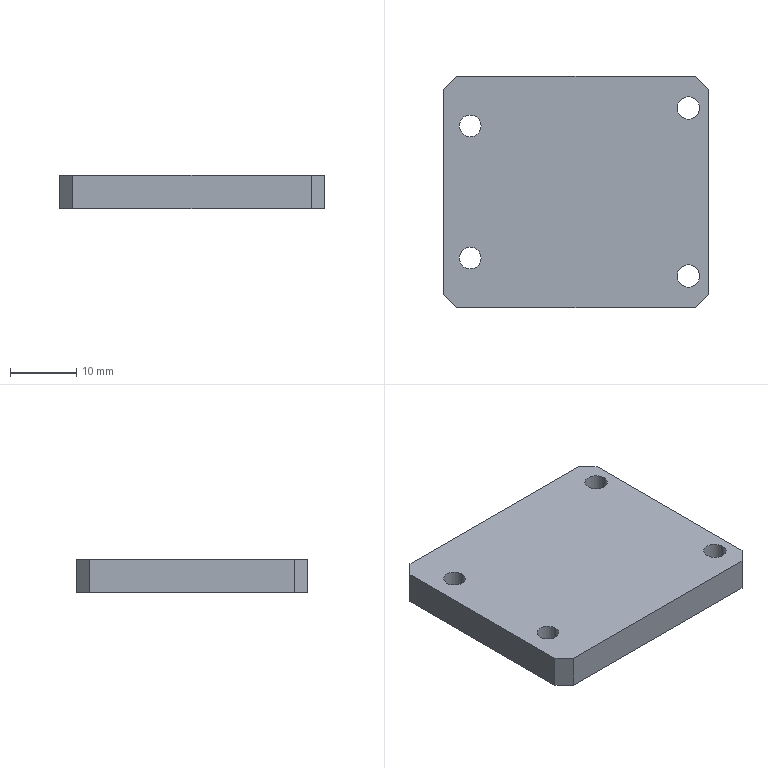Part | SolidWorks | features BaseBody 1 | 1 solid | 18 faces | box 40 x 35 x 5 mm | volume 6784 mm3 | plane 10 | cylinder 8 | commonest cylinder face diameters 3.3 x4 3.4 x4
STEP:
#1=CARTESIAN_POINT('',(18.7,12.7,5.));
#2=VERTEX_POINT('',#1);
#3=CARTESIAN_POINT('',(15.3,12.7,5.));
#4=VERTEX_POINT('',#3);
#5=CARTESIAN_POINT('',(17.,12.7,5.));
#6=DIRECTION('',(0.,0.,-1.));
#7=DIRECTION('',(-1.,0.,0.));
#8=AXIS2_PLACEMENT_3D('',#5,#6,#7);
#9=CIRCLE('',#8,1.7);
#10=EDGE_CURVE('',#2,#4,#9,.T.);
#11=ORIENTED_EDGE('',*,*,#10,.F.);
#12=CARTESIAN_POINT('',(18.7,12.7,0.));
#13=VERTEX_POINT('',#12);
#14=CARTESIAN_POINT('',(18.7,12.7,0.));
#15=DIRECTION('',(0.,0.,-1.));
#16=VECTOR('',#15,1000.);
#17=LINE('',#14,#16);
#18=EDGE_CURVE('',#2,#13,#17,.T.);
#19=ORIENTED_EDGE('',*,*,#18,.T.);
#20=CARTESIAN_POINT('',(15.3,12.7,0.));
#21=VERTEX_POINT('',#20);
#22=CARTESIAN_POINT('',(17.,12.7,0.));
#23=DIRECTION('',(0.,0.,-1.));
#24=DIRECTION('',(-1.,0.,0.));
#25=AXIS2_PLACEMENT_3D('',#22,#23,#24);
#26=CIRCLE('',#25,1.7);
#27=EDGE_CURVE('',#13,#21,#26,.T.);
#28=ORIENTED_EDGE('',*,*,#27,.T.);
#29=CARTESIAN_POINT('',(15.3,12.7,0.));
#30=DIRECTION('',(0.,0.,-1.));
#31=VECTOR('',#30,1000.);
#32=LINE('',#29,#31);
#33=EDGE_CURVE('',#4,#21,#32,.T.);
#34=ORIENTED_EDGE('',*,*,#33,.F.);
#35=EDGE_LOOP('',(#11,#19,#28,#34));
#36=FACE_OUTER_BOUND('',#35,.T.);
#37=CARTESIAN_POINT('',(17.,12.7,0.));
#38=DIRECTION('',(0.,0.,-1.));
#39=DIRECTION('',(-1.,0.,0.));
#40=AXIS2_PLACEMENT_3D('',#37,#38,#39);
#41=CYLINDRICAL_SURFACE('',#40,1.7);
#42=ADVANCED_FACE('',(#36),#41,.F.);
#43=CARTESIAN_POINT('',(18.7,-12.7,5.));
#44=VERTEX_POINT('',#43);
#45=CARTESIAN_POINT('',(15.3,-12.7,5.));
#46=VERTEX_POINT('',#45);
#47=CARTESIAN_POINT('',(17.,-12.7,5.));
#48=DIRECTION('',(0.,0.,-1.));
#49=DIRECTION('',(-1.,0.,0.));
#50=AXIS2_PLACEMENT_3D('',#47,#48,#49);
#51=CIRCLE('',#50,1.7);
#52=EDGE_CURVE('',#44,#46,#51,.T.);
#53=ORIENTED_EDGE('',*,*,#52,.F.);
#54=CARTESIAN_POINT('',(18.7,-12.7,0.));
#55=VERTEX_POINT('',#54);
#56=CARTESIAN_POINT('',(18.7,-12.7,0.));
#57=DIRECTION('',(0.,0.,-1.));
#58=VECTOR('',#57,1000.);
#59=LINE('',#56,#58);
#60=EDGE_CURVE('',#44,#55,#59,.T.);
#61=ORIENTED_EDGE('',*,*,#60,.T.);
#62=CARTESIAN_POINT('',(15.3,-12.7,0.));
#63=VERTEX_POINT('',#62);
#64=CARTESIAN_POINT('',(17.,-12.7,0.));
#65=DIRECTION('',(0.,0.,-1.));
#66=DIRECTION('',(-1.,0.,0.));
#67=AXIS2_PLACEMENT_3D('',#64,#65,#66);
#68=CIRCLE('',#67,1.7);
#69=EDGE_CURVE('',#55,#63,#68,.T.);
#70=ORIENTED_EDGE('',*,*,#69,.T.);
#71=CARTESIAN_POINT('',(15.3,-12.7,0.));
#72=DIRECTION('',(0.,0.,-1.));
#73=VECTOR('',#72,1000.);
#74=LINE('',#71,#73);
#75=EDGE_CURVE('',#46,#63,#74,.T.);
#76=ORIENTED_EDGE('',*,*,#75,.F.);
#77=EDGE_LOOP('',(#53,#61,#70,#76));
#78=FACE_OUTER_BOUND('',#77,.T.);
#79=CARTESIAN_POINT('',(17.,-12.7,0.));
#80=DIRECTION('',(0.,0.,-1.));
#81=DIRECTION('',(-1.,0.,0.));
#82=AXIS2_PLACEMENT_3D('',#79,#80,#81);
#83=CYLINDRICAL_SURFACE('',#82,1.7);
#84=ADVANCED_FACE('',(#78),#83,.F.);
#85=CARTESIAN_POINT('',(-14.35,10.,5.));
#86=VERTEX_POINT('',#85);
#87=CARTESIAN_POINT('',(-17.65,10.,5.));
#88=VERTEX_POINT('',#87);
#89=CARTESIAN_POINT('',(-16.,10.,5.));
#90=DIRECTION('',(0.,0.,-1.));
#91=DIRECTION('',(-1.,0.,0.));
#92=AXIS2_PLACEMENT_3D('',#89,#90,#91);
#93=CIRCLE('',#92,1.65);
#94=EDGE_CURVE('',#86,#88,#93,.T.);
#95=ORIENTED_EDGE('',*,*,#94,.F.);
#96=CARTESIAN_POINT('',(-14.35,10.,0.));
#97=VERTEX_POINT('',#96);
#98=CARTESIAN_POINT('',(-14.35,10.,0.));
#99=DIRECTION('',(0.,0.,-1.));
#100=VECTOR('',#99,1000.);
#101=LINE('',#98,#100);
#102=EDGE_CURVE('',#86,#97,#101,.T.);
#103=ORIENTED_EDGE('',*,*,#102,.T.);
#104=CARTESIAN_POINT('',(-17.65,10.,0.));
#105=VERTEX_POINT('',#104);
#106=CARTESIAN_POINT('',(-16.,10.,0.));
#107=DIRECTION('',(0.,0.,-1.));
#108=DIRECTION('',(-1.,0.,0.));
#109=AXIS2_PLACEMENT_3D('',#106,#107,#108);
#110=CIRCLE('',#109,1.65);
#111=EDGE_CURVE('',#97,#105,#110,.T.);
#112=ORIENTED_EDGE('',*,*,#111,.T.);
#113=CARTESIAN_POINT('',(-17.65,10.,0.));
#114=DIRECTION('',(0.,0.,-1.));
#115=VECTOR('',#114,1000.);
#116=LINE('',#113,#115);
#117=EDGE_CURVE('',#88,#105,#116,.T.);
#118=ORIENTED_EDGE('',*,*,#117,.F.);
#119=EDGE_LOOP('',(#95,#103,#112,#118));
#120=FACE_OUTER_BOUND('',#119,.T.);
#121=CARTESIAN_POINT('',(-16.,10.,0.));
#122=DIRECTION('',(0.,0.,-1.));
#123=DIRECTION('',(-1.,0.,0.));
#124=AXIS2_PLACEMENT_3D('',#121,#122,#123);
#125=CYLINDRICAL_SURFACE('',#124,1.65);
#126=ADVANCED_FACE('',(#120),#125,.F.);
#127=CARTESIAN_POINT('',(-14.35,-10.,5.));
#128=VERTEX_POINT('',#127);
#129=CARTESIAN_POINT('',(-17.65,-10.,5.));
#130=VERTEX_POINT('',#129);
#131=CARTESIAN_POINT('',(-16.,-10.,5.));
#132=DIRECTION('',(0.,0.,-1.));
#133=DIRECTION('',(-1.,0.,0.));
#134=AXIS2_PLACEMENT_3D('',#131,#132,#133);
#135=CIRCLE('',#134,1.65);
#136=EDGE_CURVE('',#128,#130,#135,.T.);
#137=ORIENTED_EDGE('',*,*,#136,.F.);
#138=CARTESIAN_POINT('',(-14.35,-10.,0.));
#139=VERTEX_POINT('',#138);
#140=CARTESIAN_POINT('',(-14.35,-10.,0.));
#141=DIRECTION('',(0.,0.,-1.));
#142=VECTOR('',#141,1000.);
#143=LINE('',#140,#142);
#144=EDGE_CURVE('',#128,#139,#143,.T.);
#145=ORIENTED_EDGE('',*,*,#144,.T.);
#146=CARTESIAN_POINT('',(-17.65,-10.,0.));
#147=VERTEX_POINT('',#146);
#148=CARTESIAN_POINT('',(-16.,-10.,0.));
#149=DIRECTION('',(0.,0.,-1.));
#150=DIRECTION('',(-1.,0.,0.));
#151=AXIS2_PLACEMENT_3D('',#148,#149,#150);
#152=CIRCLE('',#151,1.65);
#153=EDGE_CURVE('',#139,#147,#152,.T.);
#154=ORIENTED_EDGE('',*,*,#153,.T.);
#155=CARTESIAN_POINT('',(-17.65,-10.,0.));
#156=DIRECTION('',(0.,0.,-1.));
#157=VECTOR('',#156,1000.);
#158=LINE('',#155,#157);
#159=EDGE_CURVE('',#130,#147,#158,.T.);
#160=ORIENTED_EDGE('',*,*,#159,.F.);
#161=EDGE_LOOP('',(#137,#145,#154,#160));
#162=FACE_OUTER_BOUND('',#161,.T.);
#163=CARTESIAN_POINT('',(-16.,-10.,0.));
#164=DIRECTION('',(0.,0.,-1.));
#165=DIRECTION('',(-1.,0.,0.));
#166=AXIS2_PLACEMENT_3D('',#163,#164,#165);
#167=CYLINDRICAL_SURFACE('',#166,1.65);
#168=ADVANCED_FACE('',(#162),#167,.F.);
#169=CARTESIAN_POINT('',(-20.,15.5,0.));
#170=VERTEX_POINT('',#169);
#171=CARTESIAN_POINT('',(-20.,-15.5,0.));
#172=VERTEX_POINT('',#171);
#173=CARTESIAN_POINT('',(-20.,17.5,0.));
#174=DIRECTION('',(0.,-1.,0.));
#175=VECTOR('',#174,1000.);
#176=LINE('',#173,#175);
#177=EDGE_CURVE('',#170,#172,#176,.T.);
#178=ORIENTED_EDGE('',*,*,#177,.T.);
#179=CARTESIAN_POINT('',(-20.,-15.5,5.));
#180=VERTEX_POINT('',#179);
#181=CARTESIAN_POINT('',(-20.,-15.5,5.));
#182=DIRECTION('',(0.,0.,1.));
#183=VECTOR('',#182,1000.);
#184=LINE('',#181,#183);
#185=EDGE_CURVE('',#172,#180,#184,.T.);
#186=ORIENTED_EDGE('',*,*,#185,.T.);
#187=CARTESIAN_POINT('',(-20.,15.5,5.));
#188=VERTEX_POINT('',#187);
#189=CARTESIAN_POINT('',(-20.,17.5,5.));
#190=DIRECTION('',(0.,-1.,0.));
#191=VECTOR('',#190,1000.);
#192=LINE('',#189,#191);
#193=EDGE_CURVE('',#188,#180,#192,.T.);
#194=ORIENTED_EDGE('',*,*,#193,.F.);
#195=CARTESIAN_POINT('',(-20.,15.5,5.));
#196=DIRECTION('',(0.,0.,-1.));
#197=VECTOR('',#196,1000.);
#198=LINE('',#195,#197);
#199=EDGE_CURVE('',#188,#170,#198,.T.);
#200=ORIENTED_EDGE('',*,*,#199,.T.);
#201=EDGE_LOOP('',(#178,#186,#194,#200));
#202=FACE_OUTER_BOUND('',#201,.T.);
#203=CARTESIAN_POINT('',(-20.,17.5,5.));
#204=DIRECTION('',(1.,0.,0.));
#205=DIRECTION('',(0.,1.,0.));
#206=AXIS2_PLACEMENT_3D('',#203,#204,#205);
#207=PLANE('',#206);
#208=ADVANCED_FACE('',(#202),#207,.F.);
#209=CARTESIAN_POINT('',(-18.,-17.5,0.));
#210=VERTEX_POINT('',#209);
#211=CARTESIAN_POINT('',(18.,-17.5,0.));
#212=VERTEX_POINT('',#211);
#213=CARTESIAN_POINT('',(20.,-17.5,0.));
#214=DIRECTION('',(1.,0.,0.));
#215=VECTOR('',#214,1000.);
#216=LINE('',#213,#215);
#217=EDGE_CURVE('',#210,#212,#216,.T.);
#218=ORIENTED_EDGE('',*,*,#217,.T.);
#219=CARTESIAN_POINT('',(18.,-17.5,5.));
#220=VERTEX_POINT('',#219);
#221=CARTESIAN_POINT('',(18.,-17.5,5.));
#222=DIRECTION('',(0.,0.,1.));
#223=VECTOR('',#222,1000.);
#224=LINE('',#221,#223);
#225=EDGE_CURVE('',#212,#220,#224,.T.);
#226=ORIENTED_EDGE('',*,*,#225,.T.);
#227=CARTESIAN_POINT('',(-18.,-17.5,5.));
#228=VERTEX_POINT('',#227);
#229=CARTESIAN_POINT('',(20.,-17.5,5.));
#230=DIRECTION('',(1.,0.,0.));
#231=VECTOR('',#230,1000.);
#232=LINE('',#229,#231);
#233=EDGE_CURVE('',#228,#220,#232,.T.);
#234=ORIENTED_EDGE('',*,*,#233,.F.);
#235=CARTESIAN_POINT('',(-18.,-17.5,5.));
#236=DIRECTION('',(0.,0.,-1.));
#237=VECTOR('',#236,1000.);
#238=LINE('',#235,#237);
#239=EDGE_CURVE('',#228,#210,#238,.T.);
#240=ORIENTED_EDGE('',*,*,#239,.T.);
#241=EDGE_LOOP('',(#218,#226,#234,#240));
#242=FACE_OUTER_BOUND('',#241,.T.);
#243=CARTESIAN_POINT('',(20.,-17.5,5.));
#244=DIRECTION('',(0.,1.,0.));
#245=DIRECTION('',(-1.,0.,0.));
#246=AXIS2_PLACEMENT_3D('',#243,#244,#245);
#247=PLANE('',#246);
#248=ADVANCED_FACE('',(#242),#247,.F.);
#249=CARTESIAN_POINT('',(20.,-15.5,5.));
#250=VERTEX_POINT('',#249);
#251=CARTESIAN_POINT('',(20.,15.5,5.));
#252=VERTEX_POINT('',#251);
#253=CARTESIAN_POINT('',(20.,17.5,5.));
#254=DIRECTION('',(0.,1.,0.));
#255=VECTOR('',#254,1000.);
#256=LINE('',#253,#255);
#257=EDGE_CURVE('',#250,#252,#256,.T.);
#258=ORIENTED_EDGE('',*,*,#257,.F.);
#259=CARTESIAN_POINT('',(20.,-15.5,0.));
#260=VERTEX_POINT('',#259);
#261=CARTESIAN_POINT('',(20.,-15.5,5.));
#262=DIRECTION('',(0.,0.,-1.));
#263=VECTOR('',#262,1000.);
#264=LINE('',#261,#263);
#265=EDGE_CURVE('',#250,#260,#264,.T.);
#266=ORIENTED_EDGE('',*,*,#265,.T.);
#267=CARTESIAN_POINT('',(20.,15.5,0.));
#268=VERTEX_POINT('',#267);
#269=CARTESIAN_POINT('',(20.,17.5,0.));
#270=DIRECTION('',(0.,1.,0.));
#271=VECTOR('',#270,1000.);
#272=LINE('',#269,#271);
#273=EDGE_CURVE('',#260,#268,#272,.T.);
#274=ORIENTED_EDGE('',*,*,#273,.T.);
#275=CARTESIAN_POINT('',(20.,15.5,5.));
#276=DIRECTION('',(0.,0.,1.));
#277=VECTOR('',#276,1000.);
#278=LINE('',#275,#277);
#279=EDGE_CURVE('',#268,#252,#278,.T.);
#280=ORIENTED_EDGE('',*,*,#279,.T.);
#281=EDGE_LOOP('',(#258,#266,#274,#280));
#282=FACE_OUTER_BOUND('',#281,.T.);
#283=CARTESIAN_POINT('',(20.,17.5,5.));
#284=DIRECTION('',(-1.,0.,0.));
#285=DIRECTION('',(0.,-1.,0.));
#286=AXIS2_PLACEMENT_3D('',#283,#284,#285);
#287=PLANE('',#286);
#288=ADVANCED_FACE('',(#282),#287,.F.);
#289=CARTESIAN_POINT('',(18.,17.5,5.));
#290=VERTEX_POINT('',#289);
#291=CARTESIAN_POINT('',(-18.,17.5,5.));
#292=VERTEX_POINT('',#291);
#293=CARTESIAN_POINT('',(20.,17.5,5.));
#294=DIRECTION('',(-1.,0.,0.));
#295=VECTOR('',#294,1000.);
#296=LINE('',#293,#295);
#297=EDGE_CURVE('',#290,#292,#296,.T.);
#298=ORIENTED_EDGE('',*,*,#297,.F.);
#299=CARTESIAN_POINT('',(18.,17.5,0.));
#300=VERTEX_POINT('',#299);
#301=CARTESIAN_POINT('',(18.,17.5,5.));
#302=DIRECTION('',(0.,0.,-1.));
#303=VECTOR('',#302,1000.);
#304=LINE('',#301,#303);
#305=EDGE_CURVE('',#290,#300,#304,.T.);
#306=ORIENTED_EDGE('',*,*,#305,.T.);
#307=CARTESIAN_POINT('',(-18.,17.5,0.));
#308=VERTEX_POINT('',#307);
#309=CARTESIAN_POINT('',(20.,17.5,0.));
#310=DIRECTION('',(-1.,0.,0.));
#311=VECTOR('',#310,1000.);
#312=LINE('',#309,#311);
#313=EDGE_CURVE('',#300,#308,#312,.T.);
#314=ORIENTED_EDGE('',*,*,#313,.T.);
#315=CARTESIAN_POINT('',(-18.,17.5,5.));
#316=DIRECTION('',(0.,0.,1.));
#317=VECTOR('',#316,1000.);
#318=LINE('',#315,#317);
#319=EDGE_CURVE('',#308,#292,#318,.T.);
#320=ORIENTED_EDGE('',*,*,#319,.T.);
#321=EDGE_LOOP('',(#298,#306,#314,#320));
#322=FACE_OUTER_BOUND('',#321,.T.);
#323=CARTESIAN_POINT('',(20.,17.5,5.));
#324=DIRECTION('',(0.,-1.,0.));
#325=DIRECTION('',(1.,0.,0.));
#326=AXIS2_PLACEMENT_3D('',#323,#324,#325);
#327=PLANE('',#326);
#328=ADVANCED_FACE('',(#322),#327,.F.);
#329=CARTESIAN_POINT('',(17.,12.7,5.));
#330=DIRECTION('',(0.,0.,-1.));
#331=DIRECTION('',(-1.,0.,0.));
#332=AXIS2_PLACEMENT_3D('',#329,#330,#331);
#333=CIRCLE('',#332,1.7);
#334=EDGE_CURVE('',#4,#2,#333,.T.);
#335=ORIENTED_EDGE('',*,*,#334,.T.);
#336=ORIENTED_EDGE('',*,*,#10,.T.);
#337=EDGE_LOOP('',(#335,#336));
#338=FACE_BOUND('',#337,.T.);
#339=CARTESIAN_POINT('',(17.,-12.7,5.));
#340=DIRECTION('',(0.,0.,-1.));
#341=DIRECTION('',(-1.,0.,0.));
#342=AXIS2_PLACEMENT_3D('',#339,#340,#341);
#343=CIRCLE('',#342,1.7);
#344=EDGE_CURVE('',#46,#44,#343,.T.);
#345=ORIENTED_EDGE('',*,*,#344,.T.);
#346=ORIENTED_EDGE('',*,*,#52,.T.);
#347=EDGE_LOOP('',(#345,#346));
#348=FACE_BOUND('',#347,.T.);
#349=CARTESIAN_POINT('',(-16.,10.,5.));
#350=DIRECTION('',(0.,0.,-1.));
#351=DIRECTION('',(-1.,0.,0.));
#352=AXIS2_PLACEMENT_3D('',#349,#350,#351);
#353=CIRCLE('',#352,1.65);
#354=EDGE_CURVE('',#88,#86,#353,.T.);
#355=ORIENTED_EDGE('',*,*,#354,.T.);
#356=ORIENTED_EDGE('',*,*,#94,.T.);
#357=EDGE_LOOP('',(#355,#356));
#358=FACE_BOUND('',#357,.T.);
#359=CARTESIAN_POINT('',(-16.,-10.,5.));
#360=DIRECTION('',(0.,0.,-1.));
#361=DIRECTION('',(-1.,0.,0.));
#362=AXIS2_PLACEMENT_3D('',#359,#360,#361);
#363=CIRCLE('',#362,1.65);
#364=EDGE_CURVE('',#130,#128,#363,.T.);
#365=ORIENTED_EDGE('',*,*,#364,.T.);
#366=ORIENTED_EDGE('',*,*,#136,.T.);
#367=EDGE_LOOP('',(#365,#366));
#368=FACE_BOUND('',#367,.T.);
#369=ORIENTED_EDGE('',*,*,#233,.T.);
#370=CARTESIAN_POINT('',(20.,-15.5,5.));
#371=DIRECTION('',(0.7071,0.7071,0.));
#372=VECTOR('',#371,1000.);
#373=LINE('',#370,#372);
#374=EDGE_CURVE('',#220,#250,#373,.T.);
#375=ORIENTED_EDGE('',*,*,#374,.T.);
#376=ORIENTED_EDGE('',*,*,#257,.T.);
#377=CARTESIAN_POINT('',(18.,17.5,5.));
#378=DIRECTION('',(-0.7071,0.7071,0.));
#379=VECTOR('',#378,1000.);
#380=LINE('',#377,#379);
#381=EDGE_CURVE('',#252,#290,#380,.T.);
#382=ORIENTED_EDGE('',*,*,#381,.T.);
#383=ORIENTED_EDGE('',*,*,#297,.T.);
#384=CARTESIAN_POINT('',(-20.,15.5,5.));
#385=DIRECTION('',(-0.7071,-0.7071,0.));
#386=VECTOR('',#385,1000.);
#387=LINE('',#384,#386);
#388=EDGE_CURVE('',#292,#188,#387,.T.);
#389=ORIENTED_EDGE('',*,*,#388,.T.);
#390=ORIENTED_EDGE('',*,*,#193,.T.);
#391=CARTESIAN_POINT('',(-18.,-17.5,5.));
#392=DIRECTION('',(0.7071,-0.7071,0.));
#393=VECTOR('',#392,1000.);
#394=LINE('',#391,#393);
#395=EDGE_CURVE('',#180,#228,#394,.T.);
#396=ORIENTED_EDGE('',*,*,#395,.T.);
#397=EDGE_LOOP('',(#369,#375,#376,#382,#383,#389,#390,#396));
#398=FACE_OUTER_BOUND('',#397,.T.);
#399=CARTESIAN_POINT('',(0.,0.,5.));
#400=DIRECTION('',(0.,0.,-1.));
#401=DIRECTION('',(-1.,0.,0.));
#402=AXIS2_PLACEMENT_3D('',#399,#400,#401);
#403=PLANE('',#402);
#404=ADVANCED_FACE('',(#338,#348,#358,#368,#398),#403,.F.);
#405=CARTESIAN_POINT('',(17.,12.7,0.));
#406=DIRECTION('',(0.,0.,-1.));
#407=DIRECTION('',(-1.,0.,0.));
#408=AXIS2_PLACEMENT_3D('',#405,#406,#407);
#409=CIRCLE('',#408,1.7);
#410=EDGE_CURVE('',#21,#13,#409,.T.);
#411=ORIENTED_EDGE('',*,*,#410,.F.);
#412=ORIENTED_EDGE('',*,*,#27,.F.);
#413=EDGE_LOOP('',(#411,#412));
#414=FACE_BOUND('',#413,.T.);
#415=CARTESIAN_POINT('',(17.,-12.7,0.));
#416=DIRECTION('',(0.,0.,-1.));
#417=DIRECTION('',(-1.,0.,0.));
#418=AXIS2_PLACEMENT_3D('',#415,#416,#417);
#419=CIRCLE('',#418,1.7);
#420=EDGE_CURVE('',#63,#55,#419,.T.);
#421=ORIENTED_EDGE('',*,*,#420,.F.);
#422=ORIENTED_EDGE('',*,*,#69,.F.);
#423=EDGE_LOOP('',(#421,#422));
#424=FACE_BOUND('',#423,.T.);
#425=CARTESIAN_POINT('',(-16.,10.,0.));
#426=DIRECTION('',(0.,0.,-1.));
#427=DIRECTION('',(-1.,0.,0.));
#428=AXIS2_PLACEMENT_3D('',#425,#426,#427);
#429=CIRCLE('',#428,1.65);
#430=EDGE_CURVE('',#105,#97,#429,.T.);
#431=ORIENTED_EDGE('',*,*,#430,.F.);
#432=ORIENTED_EDGE('',*,*,#111,.F.);
#433=EDGE_LOOP('',(#431,#432));
#434=FACE_BOUND('',#433,.T.);
#435=CARTESIAN_POINT('',(-16.,-10.,0.));
#436=DIRECTION('',(0.,0.,-1.));
#437=DIRECTION('',(-1.,0.,0.));
#438=AXIS2_PLACEMENT_3D('',#435,#436,#437);
#439=CIRCLE('',#438,1.65);
#440=EDGE_CURVE('',#147,#139,#439,.T.);
#441=ORIENTED_EDGE('',*,*,#440,.F.);
#442=ORIENTED_EDGE('',*,*,#153,.F.);
#443=EDGE_LOOP('',(#441,#442));
#444=FACE_BOUND('',#443,.T.);
#445=ORIENTED_EDGE('',*,*,#273,.F.);
#446=CARTESIAN_POINT('',(17.75,-17.75,0.));
#447=DIRECTION('',(-0.7071,-0.7071,0.));
#448=VECTOR('',#447,1000.);
#449=LINE('',#446,#448);
#450=EDGE_CURVE('',#260,#212,#449,.T.);
#451=ORIENTED_EDGE('',*,*,#450,.T.);
#452=ORIENTED_EDGE('',*,*,#217,.F.);
#453=CARTESIAN_POINT('',(-17.75,-17.75,0.));
#454=DIRECTION('',(-0.7071,0.7071,0.));
#455=VECTOR('',#454,1000.);
#456=LINE('',#453,#455);
#457=EDGE_CURVE('',#210,#172,#456,.T.);
#458=ORIENTED_EDGE('',*,*,#457,.T.);
#459=ORIENTED_EDGE('',*,*,#177,.F.);
#460=CARTESIAN_POINT('',(-17.75,17.75,0.));
#461=DIRECTION('',(0.7071,0.7071,0.));
#462=VECTOR('',#461,1000.);
#463=LINE('',#460,#462);
#464=EDGE_CURVE('',#170,#308,#463,.T.);
#465=ORIENTED_EDGE('',*,*,#464,.T.);
#466=ORIENTED_EDGE('',*,*,#313,.F.);
#467=CARTESIAN_POINT('',(17.75,17.75,0.));
#468=DIRECTION('',(0.7071,-0.7071,0.));
#469=VECTOR('',#468,1000.);
#470=LINE('',#467,#469);
#471=EDGE_CURVE('',#300,#268,#470,.T.);
#472=ORIENTED_EDGE('',*,*,#471,.T.);
#473=EDGE_LOOP('',(#445,#451,#452,#458,#459,#465,#466,#472));
#474=FACE_OUTER_BOUND('',#473,.T.);
#475=CARTESIAN_POINT('',(0.,0.,0.));
#476=DIRECTION('',(0.,0.,-1.));
#477=DIRECTION('',(-1.,0.,0.));
#478=AXIS2_PLACEMENT_3D('',#475,#476,#477);
#479=PLANE('',#478);
#480=ADVANCED_FACE('',(#414,#424,#434,#444,#474),#479,.T.);
#481=ORIENTED_EDGE('',*,*,#144,.F.);
#482=ORIENTED_EDGE('',*,*,#364,.F.);
#483=ORIENTED_EDGE('',*,*,#159,.T.);
#484=ORIENTED_EDGE('',*,*,#440,.T.);
#485=EDGE_LOOP('',(#481,#482,#483,#484));
#486=FACE_OUTER_BOUND('',#485,.T.);
#487=CARTESIAN_POINT('',(-16.,-10.,0.));
#488=DIRECTION('',(0.,0.,-1.));
#489=DIRECTION('',(-1.,0.,0.));
#490=AXIS2_PLACEMENT_3D('',#487,#488,#489);
#491=CYLINDRICAL_SURFACE('',#490,1.65);
#492=ADVANCED_FACE('',(#486),#491,.F.);
#493=ORIENTED_EDGE('',*,*,#102,.F.);
#494=ORIENTED_EDGE('',*,*,#354,.F.);
#495=ORIENTED_EDGE('',*,*,#117,.T.);
#496=ORIENTED_EDGE('',*,*,#430,.T.);
#497=EDGE_LOOP('',(#493,#494,#495,#496));
#498=FACE_OUTER_BOUND('',#497,.T.);
#499=CARTESIAN_POINT('',(-16.,10.,0.));
#500=DIRECTION('',(0.,0.,-1.));
#501=DIRECTION('',(-1.,0.,0.));
#502=AXIS2_PLACEMENT_3D('',#499,#500,#501);
#503=CYLINDRICAL_SURFACE('',#502,1.65);
#504=ADVANCED_FACE('',(#498),#503,.F.);
#505=ORIENTED_EDGE('',*,*,#60,.F.);
#506=ORIENTED_EDGE('',*,*,#344,.F.);
#507=ORIENTED_EDGE('',*,*,#75,.T.);
#508=ORIENTED_EDGE('',*,*,#420,.T.);
#509=EDGE_LOOP('',(#505,#506,#507,#508));
#510=FACE_OUTER_BOUND('',#509,.T.);
#511=CARTESIAN_POINT('',(17.,-12.7,0.));
#512=DIRECTION('',(0.,0.,-1.));
#513=DIRECTION('',(-1.,0.,0.));
#514=AXIS2_PLACEMENT_3D('',#511,#512,#513);
#515=CYLINDRICAL_SURFACE('',#514,1.7);
#516=ADVANCED_FACE('',(#510),#515,.F.);
#517=ORIENTED_EDGE('',*,*,#18,.F.);
#518=ORIENTED_EDGE('',*,*,#334,.F.);
#519=ORIENTED_EDGE('',*,*,#33,.T.);
#520=ORIENTED_EDGE('',*,*,#410,.T.);
#521=EDGE_LOOP('',(#517,#518,#519,#520));
#522=FACE_OUTER_BOUND('',#521,.T.);
#523=CARTESIAN_POINT('',(17.,12.7,0.));
#524=DIRECTION('',(0.,0.,-1.));
#525=DIRECTION('',(-1.,0.,0.));
#526=AXIS2_PLACEMENT_3D('',#523,#524,#525);
#527=CYLINDRICAL_SURFACE('',#526,1.7);
#528=ADVANCED_FACE('',(#522),#527,.F.);
#529=ORIENTED_EDGE('',*,*,#374,.F.);
#530=ORIENTED_EDGE('',*,*,#225,.F.);
#531=ORIENTED_EDGE('',*,*,#450,.F.);
#532=ORIENTED_EDGE('',*,*,#265,.F.);
#533=EDGE_LOOP('',(#529,#530,#531,#532));
#534=FACE_OUTER_BOUND('',#533,.T.);
#535=CARTESIAN_POINT('',(20.,-15.5,5.));
#536=DIRECTION('',(-0.7071,0.7071,0.));
#537=DIRECTION('',(0.,0.,-1.));
#538=AXIS2_PLACEMENT_3D('',#535,#536,#537);
#539=PLANE('',#538);
#540=ADVANCED_FACE('',(#534),#539,.F.);
#541=ORIENTED_EDGE('',*,*,#381,.F.);
#542=ORIENTED_EDGE('',*,*,#279,.F.);
#543=ORIENTED_EDGE('',*,*,#471,.F.);
#544=ORIENTED_EDGE('',*,*,#305,.F.);
#545=EDGE_LOOP('',(#541,#542,#543,#544));
#546=FACE_OUTER_BOUND('',#545,.T.);
#547=CARTESIAN_POINT('',(18.,17.5,5.));
#548=DIRECTION('',(-0.7071,-0.7071,0.));
#549=DIRECTION('',(0.,0.,-1.));
#550=AXIS2_PLACEMENT_3D('',#547,#548,#549);
#551=PLANE('',#550);
#552=ADVANCED_FACE('',(#546),#551,.F.);
#553=ORIENTED_EDGE('',*,*,#395,.F.);
#554=ORIENTED_EDGE('',*,*,#185,.F.);
#555=ORIENTED_EDGE('',*,*,#457,.F.);
#556=ORIENTED_EDGE('',*,*,#239,.F.);
#557=EDGE_LOOP('',(#553,#554,#555,#556));
#558=FACE_OUTER_BOUND('',#557,.T.);
#559=CARTESIAN_POINT('',(-18.,-17.5,5.));
#560=DIRECTION('',(0.7071,0.7071,0.));
#561=DIRECTION('',(0.,0.,-1.));
#562=AXIS2_PLACEMENT_3D('',#559,#560,#561);
#563=PLANE('',#562);
#564=ADVANCED_FACE('',(#558),#563,.F.);
#565=ORIENTED_EDGE('',*,*,#388,.F.);
#566=ORIENTED_EDGE('',*,*,#319,.F.);
#567=ORIENTED_EDGE('',*,*,#464,.F.);
#568=ORIENTED_EDGE('',*,*,#199,.F.);
#569=EDGE_LOOP('',(#565,#566,#567,#568));
#570=FACE_OUTER_BOUND('',#569,.T.);
#571=CARTESIAN_POINT('',(-20.,15.5,5.));
#572=DIRECTION('',(0.7071,-0.7071,0.));
#573=DIRECTION('',(0.,0.,-1.));
#574=AXIS2_PLACEMENT_3D('',#571,#572,#573);
#575=PLANE('',#574);
#576=ADVANCED_FACE('',(#570),#575,.F.);
#577=CLOSED_SHELL('',(#42,#84,#126,#168,#208,#248,#288,#328,#404,#480,#492,#504,#516,#528,#540,#552,#564,#576));
#578=MANIFOLD_SOLID_BREP('',#577);
#579=CARTESIAN_POINT('',(0.,0.,0.));
#580=DIRECTION('',(0.,0.,1.));
#581=DIRECTION('',(1.,0.,0.));
#582=AXIS2_PLACEMENT_3D('',#579,#580,#581);
#583=(LENGTH_UNIT()NAMED_UNIT(*)SI_UNIT(.MILLI.,.METRE.));
#584=UNCERTAINTY_MEASURE_WITH_UNIT(LENGTH_MEASURE(0.00001),#583,'','');
#585=(NAMED_UNIT(*)PLANE_ANGLE_UNIT()SI_UNIT($,.RADIAN.));
#586=(NAMED_UNIT(*)SI_UNIT($,.STERADIAN.)SOLID_ANGLE_UNIT());
#587=(GEOMETRIC_REPRESENTATION_CONTEXT(3)GLOBAL_UNCERTAINTY_ASSIGNED_CONTEXT((#584))GLOBAL_UNIT_ASSIGNED_CONTEXT((#583,#585,#586))REPRESENTATION_CONTEXT('',''));
#588=ADVANCED_BREP_SHAPE_REPRESENTATION('',(#578,#582),#587);